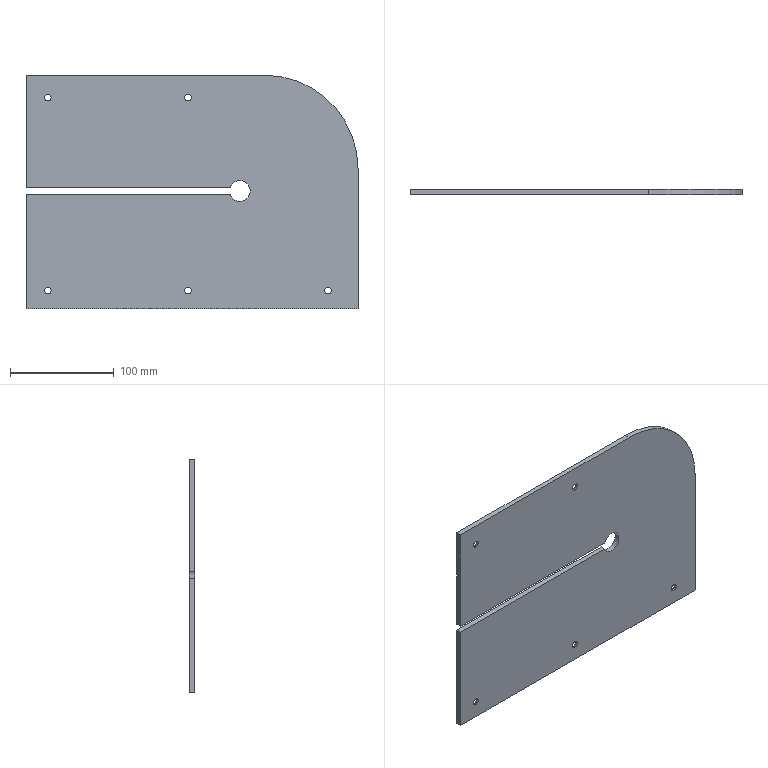Part | NX | features BREP 1 | 1 solid | 21 faces | box 320 x 5 x 225 mm | volume 341371 mm3 | plane 9 | cylinder 7 | cone 5 | commonest cylinder face diameters 6.5 x5 20 x1 180 x1
STEP:
#1=CARTESIAN_POINT('',(21.,5.,-15.1));
#2=VERTEX_POINT('',#1);
#3=CARTESIAN_POINT('',(21.,5.,-21.5));
#4=DIRECTION('',(0.,1.,0.));
#5=DIRECTION('',(0.,0.,1.));
#6=AXIS2_PLACEMENT_3D('',#3,#4,#5);
#7=CIRCLE('',#6,6.4);
#8=EDGE_CURVE('',#2,#2,#7,.T.);
#9=ORIENTED_EDGE('',*,*,#8,.T.);
#10=EDGE_LOOP('',(#9));
#11=FACE_BOUND('',#10,.T.);
#12=CARTESIAN_POINT('',(21.,1.85,-18.25));
#13=VERTEX_POINT('',#12);
#14=CARTESIAN_POINT('',(21.,1.85,-21.5));
#15=DIRECTION('',(0.,1.,0.));
#16=DIRECTION('',(0.,0.,1.));
#17=AXIS2_PLACEMENT_3D('',#14,#15,#16);
#18=CIRCLE('',#17,3.25);
#19=EDGE_CURVE('',#13,#13,#18,.T.);
#20=ORIENTED_EDGE('',*,*,#19,.F.);
#21=EDGE_LOOP('',(#20));
#22=FACE_BOUND('',#21,.T.);
#23=CARTESIAN_POINT('',(21.,5.,-21.5));
#24=DIRECTION('',(0.,1.,0.));
#25=DIRECTION('',(0.,0.,1.));
#26=AXIS2_PLACEMENT_3D('',#23,#24,#25);
#27=CONICAL_SURFACE('',#26,6.4,0.7854);
#28=ADVANCED_FACE('',(#11,#22),#27,.F.);
#29=ORIENTED_EDGE('',*,*,#19,.T.);
#30=EDGE_LOOP('',(#29));
#31=FACE_BOUND('',#30,.T.);
#32=CARTESIAN_POINT('',(21.,0.,-18.25));
#33=VERTEX_POINT('',#32);
#34=CARTESIAN_POINT('',(21.,0.,-21.5));
#35=DIRECTION('',(0.,1.,0.));
#36=DIRECTION('',(0.,0.,1.));
#37=AXIS2_PLACEMENT_3D('',#34,#35,#36);
#38=CIRCLE('',#37,3.25);
#39=EDGE_CURVE('',#33,#33,#38,.T.);
#40=ORIENTED_EDGE('',*,*,#39,.F.);
#41=EDGE_LOOP('',(#40));
#42=FACE_BOUND('',#41,.T.);
#43=CARTESIAN_POINT('',(21.,5.,-21.5));
#44=DIRECTION('',(0.,1.,0.));
#45=DIRECTION('',(0.,0.,1.));
#46=AXIS2_PLACEMENT_3D('',#43,#44,#45);
#47=CYLINDRICAL_SURFACE('',#46,3.25);
#48=ADVANCED_FACE('',(#31,#42),#47,.F.);
#49=CARTESIAN_POINT('',(156.,5.,-15.1));
#50=VERTEX_POINT('',#49);
#51=CARTESIAN_POINT('',(156.,5.,-21.5));
#52=DIRECTION('',(0.,1.,0.));
#53=DIRECTION('',(0.,0.,1.));
#54=AXIS2_PLACEMENT_3D('',#51,#52,#53);
#55=CIRCLE('',#54,6.4);
#56=EDGE_CURVE('',#50,#50,#55,.T.);
#57=ORIENTED_EDGE('',*,*,#56,.T.);
#58=EDGE_LOOP('',(#57));
#59=FACE_BOUND('',#58,.T.);
#60=CARTESIAN_POINT('',(156.,1.85,-18.25));
#61=VERTEX_POINT('',#60);
#62=CARTESIAN_POINT('',(156.,1.85,-21.5));
#63=DIRECTION('',(0.,1.,0.));
#64=DIRECTION('',(0.,0.,1.));
#65=AXIS2_PLACEMENT_3D('',#62,#63,#64);
#66=CIRCLE('',#65,3.25);
#67=EDGE_CURVE('',#61,#61,#66,.T.);
#68=ORIENTED_EDGE('',*,*,#67,.F.);
#69=EDGE_LOOP('',(#68));
#70=FACE_BOUND('',#69,.T.);
#71=CARTESIAN_POINT('',(156.,5.,-21.5));
#72=DIRECTION('',(0.,1.,0.));
#73=DIRECTION('',(0.,0.,1.));
#74=AXIS2_PLACEMENT_3D('',#71,#72,#73);
#75=CONICAL_SURFACE('',#74,6.4,0.7854);
#76=ADVANCED_FACE('',(#59,#70),#75,.F.);
#77=ORIENTED_EDGE('',*,*,#67,.T.);
#78=EDGE_LOOP('',(#77));
#79=FACE_BOUND('',#78,.T.);
#80=CARTESIAN_POINT('',(156.,0.,-18.25));
#81=VERTEX_POINT('',#80);
#82=CARTESIAN_POINT('',(156.,0.,-21.5));
#83=DIRECTION('',(0.,1.,0.));
#84=DIRECTION('',(0.,0.,1.));
#85=AXIS2_PLACEMENT_3D('',#82,#83,#84);
#86=CIRCLE('',#85,3.25);
#87=EDGE_CURVE('',#81,#81,#86,.T.);
#88=ORIENTED_EDGE('',*,*,#87,.F.);
#89=EDGE_LOOP('',(#88));
#90=FACE_BOUND('',#89,.T.);
#91=CARTESIAN_POINT('',(156.,5.,-21.5));
#92=DIRECTION('',(0.,1.,0.));
#93=DIRECTION('',(0.,0.,1.));
#94=AXIS2_PLACEMENT_3D('',#91,#92,#93);
#95=CYLINDRICAL_SURFACE('',#94,3.25);
#96=ADVANCED_FACE('',(#79,#90),#95,.F.);
#97=CARTESIAN_POINT('',(156.,5.,-201.1));
#98=VERTEX_POINT('',#97);
#99=CARTESIAN_POINT('',(156.,5.,-207.5));
#100=DIRECTION('',(0.,1.,0.));
#101=DIRECTION('',(0.,0.,1.));
#102=AXIS2_PLACEMENT_3D('',#99,#100,#101);
#103=CIRCLE('',#102,6.4);
#104=EDGE_CURVE('',#98,#98,#103,.T.);
#105=ORIENTED_EDGE('',*,*,#104,.T.);
#106=EDGE_LOOP('',(#105));
#107=FACE_BOUND('',#106,.T.);
#108=CARTESIAN_POINT('',(156.,1.85,-204.25));
#109=VERTEX_POINT('',#108);
#110=CARTESIAN_POINT('',(156.,1.85,-207.5));
#111=DIRECTION('',(0.,1.,0.));
#112=DIRECTION('',(0.,0.,1.));
#113=AXIS2_PLACEMENT_3D('',#110,#111,#112);
#114=CIRCLE('',#113,3.25);
#115=EDGE_CURVE('',#109,#109,#114,.T.);
#116=ORIENTED_EDGE('',*,*,#115,.F.);
#117=EDGE_LOOP('',(#116));
#118=FACE_BOUND('',#117,.T.);
#119=CARTESIAN_POINT('',(156.,5.,-207.5));
#120=DIRECTION('',(0.,1.,0.));
#121=DIRECTION('',(0.,0.,1.));
#122=AXIS2_PLACEMENT_3D('',#119,#120,#121);
#123=CONICAL_SURFACE('',#122,6.4,0.7854);
#124=ADVANCED_FACE('',(#107,#118),#123,.F.);
#125=ORIENTED_EDGE('',*,*,#115,.T.);
#126=EDGE_LOOP('',(#125));
#127=FACE_BOUND('',#126,.T.);
#128=CARTESIAN_POINT('',(156.,0.,-204.25));
#129=VERTEX_POINT('',#128);
#130=CARTESIAN_POINT('',(156.,0.,-207.5));
#131=DIRECTION('',(0.,1.,0.));
#132=DIRECTION('',(0.,0.,1.));
#133=AXIS2_PLACEMENT_3D('',#130,#131,#132);
#134=CIRCLE('',#133,3.25);
#135=EDGE_CURVE('',#129,#129,#134,.T.);
#136=ORIENTED_EDGE('',*,*,#135,.F.);
#137=EDGE_LOOP('',(#136));
#138=FACE_BOUND('',#137,.T.);
#139=CARTESIAN_POINT('',(156.,5.,-207.5));
#140=DIRECTION('',(0.,1.,0.));
#141=DIRECTION('',(0.,0.,1.));
#142=AXIS2_PLACEMENT_3D('',#139,#140,#141);
#143=CYLINDRICAL_SURFACE('',#142,3.25);
#144=ADVANCED_FACE('',(#127,#138),#143,.F.);
#145=CARTESIAN_POINT('',(291.,5.,-201.1));
#146=VERTEX_POINT('',#145);
#147=CARTESIAN_POINT('',(291.,5.,-207.5));
#148=DIRECTION('',(0.,1.,0.));
#149=DIRECTION('',(0.,0.,1.));
#150=AXIS2_PLACEMENT_3D('',#147,#148,#149);
#151=CIRCLE('',#150,6.4);
#152=EDGE_CURVE('',#146,#146,#151,.T.);
#153=ORIENTED_EDGE('',*,*,#152,.T.);
#154=EDGE_LOOP('',(#153));
#155=FACE_BOUND('',#154,.T.);
#156=CARTESIAN_POINT('',(291.,1.85,-204.25));
#157=VERTEX_POINT('',#156);
#158=CARTESIAN_POINT('',(291.,1.85,-207.5));
#159=DIRECTION('',(0.,1.,0.));
#160=DIRECTION('',(0.,0.,1.));
#161=AXIS2_PLACEMENT_3D('',#158,#159,#160);
#162=CIRCLE('',#161,3.25);
#163=EDGE_CURVE('',#157,#157,#162,.T.);
#164=ORIENTED_EDGE('',*,*,#163,.F.);
#165=EDGE_LOOP('',(#164));
#166=FACE_BOUND('',#165,.T.);
#167=CARTESIAN_POINT('',(291.,5.,-207.5));
#168=DIRECTION('',(0.,1.,0.));
#169=DIRECTION('',(0.,0.,1.));
#170=AXIS2_PLACEMENT_3D('',#167,#168,#169);
#171=CONICAL_SURFACE('',#170,6.4,0.7854);
#172=ADVANCED_FACE('',(#155,#166),#171,.F.);
#173=ORIENTED_EDGE('',*,*,#163,.T.);
#174=EDGE_LOOP('',(#173));
#175=FACE_BOUND('',#174,.T.);
#176=CARTESIAN_POINT('',(291.,0.,-204.25));
#177=VERTEX_POINT('',#176);
#178=CARTESIAN_POINT('',(291.,0.,-207.5));
#179=DIRECTION('',(0.,1.,0.));
#180=DIRECTION('',(0.,0.,1.));
#181=AXIS2_PLACEMENT_3D('',#178,#179,#180);
#182=CIRCLE('',#181,3.25);
#183=EDGE_CURVE('',#177,#177,#182,.T.);
#184=ORIENTED_EDGE('',*,*,#183,.F.);
#185=EDGE_LOOP('',(#184));
#186=FACE_BOUND('',#185,.T.);
#187=CARTESIAN_POINT('',(291.,5.,-207.5));
#188=DIRECTION('',(0.,1.,0.));
#189=DIRECTION('',(0.,0.,1.));
#190=AXIS2_PLACEMENT_3D('',#187,#188,#189);
#191=CYLINDRICAL_SURFACE('',#190,3.25);
#192=ADVANCED_FACE('',(#175,#186),#191,.F.);
#193=CARTESIAN_POINT('',(21.,5.,-201.1));
#194=VERTEX_POINT('',#193);
#195=CARTESIAN_POINT('',(21.,5.,-207.5));
#196=DIRECTION('',(0.,1.,0.));
#197=DIRECTION('',(0.,0.,1.));
#198=AXIS2_PLACEMENT_3D('',#195,#196,#197);
#199=CIRCLE('',#198,6.4);
#200=EDGE_CURVE('',#194,#194,#199,.T.);
#201=ORIENTED_EDGE('',*,*,#200,.T.);
#202=EDGE_LOOP('',(#201));
#203=FACE_BOUND('',#202,.T.);
#204=CARTESIAN_POINT('',(21.,1.85,-204.25));
#205=VERTEX_POINT('',#204);
#206=CARTESIAN_POINT('',(21.,1.85,-207.5));
#207=DIRECTION('',(0.,1.,0.));
#208=DIRECTION('',(0.,0.,1.));
#209=AXIS2_PLACEMENT_3D('',#206,#207,#208);
#210=CIRCLE('',#209,3.25);
#211=EDGE_CURVE('',#205,#205,#210,.T.);
#212=ORIENTED_EDGE('',*,*,#211,.F.);
#213=EDGE_LOOP('',(#212));
#214=FACE_BOUND('',#213,.T.);
#215=CARTESIAN_POINT('',(21.,5.,-207.5));
#216=DIRECTION('',(0.,1.,0.));
#217=DIRECTION('',(0.,0.,1.));
#218=AXIS2_PLACEMENT_3D('',#215,#216,#217);
#219=CONICAL_SURFACE('',#218,6.4,0.7854);
#220=ADVANCED_FACE('',(#203,#214),#219,.F.);
#221=ORIENTED_EDGE('',*,*,#211,.T.);
#222=EDGE_LOOP('',(#221));
#223=FACE_BOUND('',#222,.T.);
#224=CARTESIAN_POINT('',(21.,0.,-204.25));
#225=VERTEX_POINT('',#224);
#226=CARTESIAN_POINT('',(21.,0.,-207.5));
#227=DIRECTION('',(0.,1.,0.));
#228=DIRECTION('',(0.,0.,1.));
#229=AXIS2_PLACEMENT_3D('',#226,#227,#228);
#230=CIRCLE('',#229,3.25);
#231=EDGE_CURVE('',#225,#225,#230,.T.);
#232=ORIENTED_EDGE('',*,*,#231,.F.);
#233=EDGE_LOOP('',(#232));
#234=FACE_BOUND('',#233,.T.);
#235=CARTESIAN_POINT('',(21.,5.,-207.5));
#236=DIRECTION('',(0.,1.,0.));
#237=DIRECTION('',(0.,0.,1.));
#238=AXIS2_PLACEMENT_3D('',#235,#236,#237);
#239=CYLINDRICAL_SURFACE('',#238,3.25);
#240=ADVANCED_FACE('',(#223,#234),#239,.F.);
#241=CARTESIAN_POINT('',(196.633,0.,-115.));
#242=VERTEX_POINT('',#241);
#243=CARTESIAN_POINT('',(196.633,0.,-108.));
#244=VERTEX_POINT('',#243);
#245=CARTESIAN_POINT('',(206.,0.,-111.5));
#246=DIRECTION('',(0.,-1.,0.));
#247=DIRECTION('',(0.,0.,-1.));
#248=AXIS2_PLACEMENT_3D('',#245,#246,#247);
#249=CIRCLE('',#248,10.);
#250=EDGE_CURVE('',#242,#244,#249,.T.);
#251=ORIENTED_EDGE('',*,*,#250,.T.);
#252=CARTESIAN_POINT('',(196.633,5.,-108.));
#253=VERTEX_POINT('',#252);
#254=CARTESIAN_POINT('',(196.633,-5.,-108.));
#255=DIRECTION('',(0.,1.,0.));
#256=VECTOR('',#255,1000.);
#257=LINE('',#254,#256);
#258=EDGE_CURVE('',#244,#253,#257,.T.);
#259=ORIENTED_EDGE('',*,*,#258,.T.);
#260=CARTESIAN_POINT('',(196.633,5.,-115.));
#261=VERTEX_POINT('',#260);
#262=CARTESIAN_POINT('',(206.,5.,-111.5));
#263=DIRECTION('',(0.,1.,0.));
#264=DIRECTION('',(0.,0.,1.));
#265=AXIS2_PLACEMENT_3D('',#262,#263,#264);
#266=CIRCLE('',#265,10.);
#267=EDGE_CURVE('',#253,#261,#266,.T.);
#268=ORIENTED_EDGE('',*,*,#267,.T.);
#269=CARTESIAN_POINT('',(196.633,0.,-115.));
#270=DIRECTION('',(0.,-1.,0.));
#271=VECTOR('',#270,1000.);
#272=LINE('',#269,#271);
#273=EDGE_CURVE('',#261,#242,#272,.T.);
#274=ORIENTED_EDGE('',*,*,#273,.T.);
#275=EDGE_LOOP('',(#251,#259,#268,#274));
#276=FACE_BOUND('',#275,.T.);
#277=CARTESIAN_POINT('',(206.,-5.,-111.5));
#278=DIRECTION('',(0.,1.,0.));
#279=DIRECTION('',(0.,0.,1.));
#280=AXIS2_PLACEMENT_3D('',#277,#278,#279);
#281=CYLINDRICAL_SURFACE('',#280,10.);
#282=ADVANCED_FACE('',(#276),#281,.F.);
#283=CARTESIAN_POINT('',(0.,0.,-225.));
#284=VERTEX_POINT('',#283);
#285=CARTESIAN_POINT('',(0.,0.,-115.));
#286=VERTEX_POINT('',#285);
#287=CARTESIAN_POINT('',(0.,0.,0.));
#288=DIRECTION('',(0.,0.,1.));
#289=VECTOR('',#288,1000.);
#290=LINE('',#287,#289);
#291=EDGE_CURVE('',#284,#286,#290,.T.);
#292=ORIENTED_EDGE('',*,*,#291,.T.);
#293=CARTESIAN_POINT('',(0.,5.,-115.));
#294=VERTEX_POINT('',#293);
#295=CARTESIAN_POINT('',(0.,-5.,-115.));
#296=DIRECTION('',(0.,1.,0.));
#297=VECTOR('',#296,1000.);
#298=LINE('',#295,#297);
#299=EDGE_CURVE('',#286,#294,#298,.T.);
#300=ORIENTED_EDGE('',*,*,#299,.T.);
#301=CARTESIAN_POINT('',(0.,5.,-225.));
#302=VERTEX_POINT('',#301);
#303=CARTESIAN_POINT('',(0.,5.,0.));
#304=DIRECTION('',(0.,0.,1.));
#305=VECTOR('',#304,1000.);
#306=LINE('',#303,#305);
#307=EDGE_CURVE('',#302,#294,#306,.T.);
#308=ORIENTED_EDGE('',*,*,#307,.F.);
#309=CARTESIAN_POINT('',(0.,5.,-225.));
#310=DIRECTION('',(0.,-1.,0.));
#311=VECTOR('',#310,1000.);
#312=LINE('',#309,#311);
#313=EDGE_CURVE('',#302,#284,#312,.T.);
#314=ORIENTED_EDGE('',*,*,#313,.T.);
#315=EDGE_LOOP('',(#292,#300,#308,#314));
#316=FACE_BOUND('',#315,.T.);
#317=CARTESIAN_POINT('',(0.,5.,0.));
#318=DIRECTION('',(1.,0.,0.));
#319=DIRECTION('',(0.,0.,-1.));
#320=AXIS2_PLACEMENT_3D('',#317,#318,#319);
#321=PLANE('',#320);
#322=ADVANCED_FACE('',(#316),#321,.F.);
#323=CARTESIAN_POINT('',(0.,5.,-108.));
#324=VERTEX_POINT('',#323);
#325=CARTESIAN_POINT('',(0.,5.,0.));
#326=VERTEX_POINT('',#325);
#327=CARTESIAN_POINT('',(0.,5.,0.));
#328=DIRECTION('',(0.,0.,1.));
#329=VECTOR('',#328,1000.);
#330=LINE('',#327,#329);
#331=EDGE_CURVE('',#324,#326,#330,.T.);
#332=ORIENTED_EDGE('',*,*,#331,.F.);
#333=CARTESIAN_POINT('',(0.,0.,-108.));
#334=VERTEX_POINT('',#333);
#335=CARTESIAN_POINT('',(0.,-5.,-108.));
#336=DIRECTION('',(0.,1.,0.));
#337=VECTOR('',#336,1000.);
#338=LINE('',#335,#337);
#339=EDGE_CURVE('',#334,#324,#338,.T.);
#340=ORIENTED_EDGE('',*,*,#339,.F.);
#341=CARTESIAN_POINT('',(0.,0.,0.));
#342=VERTEX_POINT('',#341);
#343=CARTESIAN_POINT('',(0.,0.,0.));
#344=DIRECTION('',(0.,0.,1.));
#345=VECTOR('',#344,1000.);
#346=LINE('',#343,#345);
#347=EDGE_CURVE('',#334,#342,#346,.T.);
#348=ORIENTED_EDGE('',*,*,#347,.T.);
#349=CARTESIAN_POINT('',(0.,5.,0.));
#350=DIRECTION('',(0.,-1.,0.));
#351=VECTOR('',#350,1000.);
#352=LINE('',#349,#351);
#353=EDGE_CURVE('',#326,#342,#352,.T.);
#354=ORIENTED_EDGE('',*,*,#353,.F.);
#355=EDGE_LOOP('',(#332,#340,#348,#354));
#356=FACE_BOUND('',#355,.T.);
#357=CARTESIAN_POINT('',(0.,5.,0.));
#358=DIRECTION('',(1.,0.,0.));
#359=DIRECTION('',(0.,0.,-1.));
#360=AXIS2_PLACEMENT_3D('',#357,#358,#359);
#361=PLANE('',#360);
#362=ADVANCED_FACE('',(#356),#361,.F.);
#363=CARTESIAN_POINT('',(230.,0.,0.));
#364=VERTEX_POINT('',#363);
#365=CARTESIAN_POINT('',(0.,0.,0.));
#366=DIRECTION('',(1.,0.,0.));
#367=VECTOR('',#366,1000.);
#368=LINE('',#365,#367);
#369=EDGE_CURVE('',#342,#364,#368,.T.);
#370=ORIENTED_EDGE('',*,*,#369,.T.);
#371=CARTESIAN_POINT('',(230.,5.,0.));
#372=VERTEX_POINT('',#371);
#373=CARTESIAN_POINT('',(230.,5.,0.));
#374=DIRECTION('',(0.,-1.,0.));
#375=VECTOR('',#374,1000.);
#376=LINE('',#373,#375);
#377=EDGE_CURVE('',#372,#364,#376,.T.);
#378=ORIENTED_EDGE('',*,*,#377,.F.);
#379=CARTESIAN_POINT('',(0.,5.,0.));
#380=DIRECTION('',(1.,0.,0.));
#381=VECTOR('',#380,1000.);
#382=LINE('',#379,#381);
#383=EDGE_CURVE('',#326,#372,#382,.T.);
#384=ORIENTED_EDGE('',*,*,#383,.F.);
#385=ORIENTED_EDGE('',*,*,#353,.T.);
#386=EDGE_LOOP('',(#370,#378,#384,#385));
#387=FACE_BOUND('',#386,.T.);
#388=CARTESIAN_POINT('',(0.,5.,0.));
#389=DIRECTION('',(0.,0.,-1.));
#390=DIRECTION('',(-1.,0.,0.));
#391=AXIS2_PLACEMENT_3D('',#388,#389,#390);
#392=PLANE('',#391);
#393=ADVANCED_FACE('',(#387),#392,.F.);
#394=CARTESIAN_POINT('',(320.,0.,-90.));
#395=VERTEX_POINT('',#394);
#396=CARTESIAN_POINT('',(230.,0.,-90.));
#397=DIRECTION('',(0.,1.,0.));
#398=DIRECTION('',(0.,0.,-1.));
#399=AXIS2_PLACEMENT_3D('',#396,#397,#398);
#400=CIRCLE('',#399,90.);
#401=EDGE_CURVE('',#364,#395,#400,.T.);
#402=ORIENTED_EDGE('',*,*,#401,.T.);
#403=CARTESIAN_POINT('',(320.,5.,-90.));
#404=VERTEX_POINT('',#403);
#405=CARTESIAN_POINT('',(320.,5.,-90.));
#406=DIRECTION('',(0.,-1.,0.));
#407=VECTOR('',#406,1000.);
#408=LINE('',#405,#407);
#409=EDGE_CURVE('',#404,#395,#408,.T.);
#410=ORIENTED_EDGE('',*,*,#409,.F.);
#411=CARTESIAN_POINT('',(230.,5.,-90.));
#412=DIRECTION('',(0.,1.,0.));
#413=DIRECTION('',(0.,0.,-1.));
#414=AXIS2_PLACEMENT_3D('',#411,#412,#413);
#415=CIRCLE('',#414,90.);
#416=EDGE_CURVE('',#372,#404,#415,.T.);
#417=ORIENTED_EDGE('',*,*,#416,.F.);
#418=ORIENTED_EDGE('',*,*,#377,.T.);
#419=EDGE_LOOP('',(#402,#410,#417,#418));
#420=FACE_BOUND('',#419,.T.);
#421=CARTESIAN_POINT('',(230.,5.,-90.));
#422=DIRECTION('',(0.,-1.,0.));
#423=DIRECTION('',(0.,0.,-1.));
#424=AXIS2_PLACEMENT_3D('',#421,#422,#423);
#425=CYLINDRICAL_SURFACE('',#424,90.);
#426=ADVANCED_FACE('',(#420),#425,.T.);
#427=CARTESIAN_POINT('',(320.,0.,-225.));
#428=VERTEX_POINT('',#427);
#429=CARTESIAN_POINT('',(320.,0.,-90.));
#430=DIRECTION('',(0.,0.,-1.));
#431=VECTOR('',#430,1000.);
#432=LINE('',#429,#431);
#433=EDGE_CURVE('',#395,#428,#432,.T.);
#434=ORIENTED_EDGE('',*,*,#433,.T.);
#435=CARTESIAN_POINT('',(320.,5.,-225.));
#436=VERTEX_POINT('',#435);
#437=CARTESIAN_POINT('',(320.,5.,-225.));
#438=DIRECTION('',(0.,-1.,0.));
#439=VECTOR('',#438,1000.);
#440=LINE('',#437,#439);
#441=EDGE_CURVE('',#436,#428,#440,.T.);
#442=ORIENTED_EDGE('',*,*,#441,.F.);
#443=CARTESIAN_POINT('',(320.,5.,-90.));
#444=DIRECTION('',(0.,0.,-1.));
#445=VECTOR('',#444,1000.);
#446=LINE('',#443,#445);
#447=EDGE_CURVE('',#404,#436,#446,.T.);
#448=ORIENTED_EDGE('',*,*,#447,.F.);
#449=ORIENTED_EDGE('',*,*,#409,.T.);
#450=EDGE_LOOP('',(#434,#442,#448,#449));
#451=FACE_BOUND('',#450,.T.);
#452=CARTESIAN_POINT('',(320.,5.,-90.));
#453=DIRECTION('',(-1.,0.,0.));
#454=DIRECTION('',(0.,0.,1.));
#455=AXIS2_PLACEMENT_3D('',#452,#453,#454);
#456=PLANE('',#455);
#457=ADVANCED_FACE('',(#451),#456,.F.);
#458=CARTESIAN_POINT('',(0.,0.,-225.));
#459=DIRECTION('',(-1.,0.,0.));
#460=VECTOR('',#459,1000.);
#461=LINE('',#458,#460);
#462=EDGE_CURVE('',#428,#284,#461,.T.);
#463=ORIENTED_EDGE('',*,*,#462,.T.);
#464=ORIENTED_EDGE('',*,*,#313,.F.);
#465=CARTESIAN_POINT('',(0.,5.,-225.));
#466=DIRECTION('',(-1.,0.,0.));
#467=VECTOR('',#466,1000.);
#468=LINE('',#465,#467);
#469=EDGE_CURVE('',#436,#302,#468,.T.);
#470=ORIENTED_EDGE('',*,*,#469,.F.);
#471=ORIENTED_EDGE('',*,*,#441,.T.);
#472=EDGE_LOOP('',(#463,#464,#470,#471));
#473=FACE_BOUND('',#472,.T.);
#474=CARTESIAN_POINT('',(0.,5.,-225.));
#475=DIRECTION('',(0.,0.,1.));
#476=DIRECTION('',(1.,0.,0.));
#477=AXIS2_PLACEMENT_3D('',#474,#475,#476);
#478=PLANE('',#477);
#479=ADVANCED_FACE('',(#473),#478,.F.);
#480=ORIENTED_EDGE('',*,*,#8,.F.);
#481=EDGE_LOOP('',(#480));
#482=FACE_BOUND('',#481,.T.);
#483=ORIENTED_EDGE('',*,*,#56,.F.);
#484=EDGE_LOOP('',(#483));
#485=FACE_BOUND('',#484,.T.);
#486=ORIENTED_EDGE('',*,*,#104,.F.);
#487=EDGE_LOOP('',(#486));
#488=FACE_BOUND('',#487,.T.);
#489=ORIENTED_EDGE('',*,*,#152,.F.);
#490=EDGE_LOOP('',(#489));
#491=FACE_BOUND('',#490,.T.);
#492=ORIENTED_EDGE('',*,*,#200,.F.);
#493=EDGE_LOOP('',(#492));
#494=FACE_BOUND('',#493,.T.);
#495=ORIENTED_EDGE('',*,*,#307,.T.);
#496=CARTESIAN_POINT('',(0.,5.,-115.));
#497=DIRECTION('',(-1.,0.,0.));
#498=VECTOR('',#497,1000.);
#499=LINE('',#496,#498);
#500=EDGE_CURVE('',#261,#294,#499,.T.);
#501=ORIENTED_EDGE('',*,*,#500,.F.);
#502=ORIENTED_EDGE('',*,*,#267,.F.);
#503=CARTESIAN_POINT('',(0.,5.,-108.));
#504=DIRECTION('',(1.,0.,0.));
#505=VECTOR('',#504,1000.);
#506=LINE('',#503,#505);
#507=EDGE_CURVE('',#324,#253,#506,.T.);
#508=ORIENTED_EDGE('',*,*,#507,.F.);
#509=ORIENTED_EDGE('',*,*,#331,.T.);
#510=ORIENTED_EDGE('',*,*,#383,.T.);
#511=ORIENTED_EDGE('',*,*,#416,.T.);
#512=ORIENTED_EDGE('',*,*,#447,.T.);
#513=ORIENTED_EDGE('',*,*,#469,.T.);
#514=EDGE_LOOP('',(#495,#501,#502,#508,#509,#510,#511,#512,#513));
#515=FACE_BOUND('',#514,.T.);
#516=CARTESIAN_POINT('',(230.,5.,-90.));
#517=DIRECTION('',(0.,-1.,0.));
#518=DIRECTION('',(0.,0.,-1.));
#519=AXIS2_PLACEMENT_3D('',#516,#517,#518);
#520=PLANE('',#519);
#521=ADVANCED_FACE('',(#482,#485,#488,#491,#494,#515),#520,.F.);
#522=CARTESIAN_POINT('',(230.,0.,-115.));
#523=DIRECTION('',(1.,0.,0.));
#524=VECTOR('',#523,1000.);
#525=LINE('',#522,#524);
#526=EDGE_CURVE('',#286,#242,#525,.T.);
#527=ORIENTED_EDGE('',*,*,#526,.F.);
#528=ORIENTED_EDGE('',*,*,#291,.F.);
#529=ORIENTED_EDGE('',*,*,#462,.F.);
#530=ORIENTED_EDGE('',*,*,#433,.F.);
#531=ORIENTED_EDGE('',*,*,#401,.F.);
#532=ORIENTED_EDGE('',*,*,#369,.F.);
#533=ORIENTED_EDGE('',*,*,#347,.F.);
#534=CARTESIAN_POINT('',(230.,0.,-108.));
#535=DIRECTION('',(-1.,0.,0.));
#536=VECTOR('',#535,1000.);
#537=LINE('',#534,#536);
#538=EDGE_CURVE('',#244,#334,#537,.T.);
#539=ORIENTED_EDGE('',*,*,#538,.F.);
#540=ORIENTED_EDGE('',*,*,#250,.F.);
#541=EDGE_LOOP('',(#527,#528,#529,#530,#531,#532,#533,#539,#540));
#542=FACE_BOUND('',#541,.T.);
#543=ORIENTED_EDGE('',*,*,#39,.T.);
#544=EDGE_LOOP('',(#543));
#545=FACE_BOUND('',#544,.T.);
#546=ORIENTED_EDGE('',*,*,#87,.T.);
#547=EDGE_LOOP('',(#546));
#548=FACE_BOUND('',#547,.T.);
#549=ORIENTED_EDGE('',*,*,#135,.T.);
#550=EDGE_LOOP('',(#549));
#551=FACE_BOUND('',#550,.T.);
#552=ORIENTED_EDGE('',*,*,#183,.T.);
#553=EDGE_LOOP('',(#552));
#554=FACE_BOUND('',#553,.T.);
#555=ORIENTED_EDGE('',*,*,#231,.T.);
#556=EDGE_LOOP('',(#555));
#557=FACE_BOUND('',#556,.T.);
#558=CARTESIAN_POINT('',(230.,0.,-90.));
#559=DIRECTION('',(0.,-1.,0.));
#560=DIRECTION('',(0.,0.,-1.));
#561=AXIS2_PLACEMENT_3D('',#558,#559,#560);
#562=PLANE('',#561);
#563=ADVANCED_FACE('',(#542,#545,#548,#551,#554,#557),#562,.T.);
#564=ORIENTED_EDGE('',*,*,#538,.T.);
#565=ORIENTED_EDGE('',*,*,#339,.T.);
#566=ORIENTED_EDGE('',*,*,#507,.T.);
#567=ORIENTED_EDGE('',*,*,#258,.F.);
#568=EDGE_LOOP('',(#564,#565,#566,#567));
#569=FACE_BOUND('',#568,.T.);
#570=CARTESIAN_POINT('',(0.,-5.,-108.));
#571=DIRECTION('',(0.,0.,1.));
#572=DIRECTION('',(1.,0.,0.));
#573=AXIS2_PLACEMENT_3D('',#570,#571,#572);
#574=PLANE('',#573);
#575=ADVANCED_FACE('',(#569),#574,.F.);
#576=ORIENTED_EDGE('',*,*,#526,.T.);
#577=ORIENTED_EDGE('',*,*,#273,.F.);
#578=ORIENTED_EDGE('',*,*,#500,.T.);
#579=ORIENTED_EDGE('',*,*,#299,.F.);
#580=EDGE_LOOP('',(#576,#577,#578,#579));
#581=FACE_BOUND('',#580,.T.);
#582=CARTESIAN_POINT('',(0.,-5.,-115.));
#583=DIRECTION('',(0.,0.,-1.));
#584=DIRECTION('',(-1.,0.,0.));
#585=AXIS2_PLACEMENT_3D('',#582,#583,#584);
#586=PLANE('',#585);
#587=ADVANCED_FACE('',(#581),#586,.F.);
#588=CLOSED_SHELL('',(#28,#48,#76,#96,#124,#144,#172,#192,#220,#240,#282,#322,#362,#393,#426,#457,#479,#521,#563,#575,#587));
#589=MANIFOLD_SOLID_BREP('',#588);
#590=(LENGTH_UNIT()NAMED_UNIT(*)SI_UNIT(.MILLI.,.METRE.));
#591=UNCERTAINTY_MEASURE_WITH_UNIT(LENGTH_MEASURE(0.00001),#590,'','');
#592=(NAMED_UNIT(*)PLANE_ANGLE_UNIT()SI_UNIT($,.RADIAN.));
#593=(NAMED_UNIT(*)SI_UNIT($,.STERADIAN.)SOLID_ANGLE_UNIT());
#594=(GEOMETRIC_REPRESENTATION_CONTEXT(3)GLOBAL_UNCERTAINTY_ASSIGNED_CONTEXT((#591))GLOBAL_UNIT_ASSIGNED_CONTEXT((#590,#592,#593))REPRESENTATION_CONTEXT('',''));
#595=ADVANCED_BREP_SHAPE_REPRESENTATION('',(#589),#594);